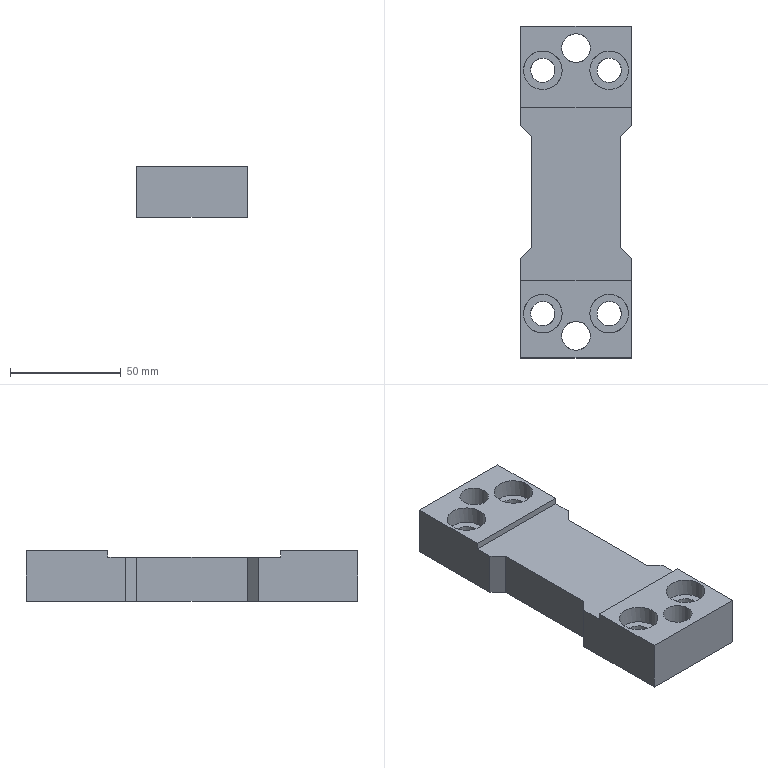Part | NX | features solid 2 | 1 solid | 32 faces | box 50 x 150 x 23 mm | volume 130295 mm3 | plane 22 | cylinder 10 | commonest cylinder face diameters 11 x4 17.5 x4 13 x2
STEP:
#1=CARTESIAN_POINT('',(-470.,-708.,-75.));
#2=VERTEX_POINT('',#1);
#3=CARTESIAN_POINT('',(-470.,-663.,-75.));
#4=VERTEX_POINT('',#3);
#5=CARTESIAN_POINT('',(-470.,-708.,-75.));
#6=DIRECTION('',(0.,1.,0.));
#7=VECTOR('',#6,1000.);
#8=LINE('',#5,#7);
#9=EDGE_CURVE('',#2,#4,#8,.T.);
#10=ORIENTED_EDGE('',*,*,#9,.F.);
#11=CARTESIAN_POINT('',(-520.,-708.,-75.));
#12=VERTEX_POINT('',#11);
#13=CARTESIAN_POINT('',(-520.,-708.,-75.));
#14=DIRECTION('',(1.,0.,0.));
#15=VECTOR('',#14,1000.);
#16=LINE('',#13,#15);
#17=EDGE_CURVE('',#12,#2,#16,.T.);
#18=ORIENTED_EDGE('',*,*,#17,.F.);
#19=CARTESIAN_POINT('',(-520.,-663.,-75.));
#20=VERTEX_POINT('',#19);
#21=CARTESIAN_POINT('',(-520.,-708.,-75.));
#22=DIRECTION('',(0.,1.,0.));
#23=VECTOR('',#22,1000.);
#24=LINE('',#21,#23);
#25=EDGE_CURVE('',#12,#20,#24,.T.);
#26=ORIENTED_EDGE('',*,*,#25,.T.);
#27=CARTESIAN_POINT('',(-515.,-658.,-75.));
#28=VERTEX_POINT('',#27);
#29=CARTESIAN_POINT('',(-515.,-658.,-75.));
#30=DIRECTION('',(-0.7071,-0.7071,0.));
#31=VECTOR('',#30,1000.);
#32=LINE('',#29,#31);
#33=EDGE_CURVE('',#28,#20,#32,.T.);
#34=ORIENTED_EDGE('',*,*,#33,.F.);
#35=CARTESIAN_POINT('',(-515.,-608.,-75.));
#36=VERTEX_POINT('',#35);
#37=CARTESIAN_POINT('',(-515.,-658.,-75.));
#38=DIRECTION('',(0.,1.,0.));
#39=VECTOR('',#38,1000.);
#40=LINE('',#37,#39);
#41=EDGE_CURVE('',#28,#36,#40,.T.);
#42=ORIENTED_EDGE('',*,*,#41,.T.);
#43=CARTESIAN_POINT('',(-520.,-603.,-75.));
#44=VERTEX_POINT('',#43);
#45=CARTESIAN_POINT('',(-515.,-608.,-75.));
#46=DIRECTION('',(-0.7071,0.7071,0.));
#47=VECTOR('',#46,1000.);
#48=LINE('',#45,#47);
#49=EDGE_CURVE('',#36,#44,#48,.T.);
#50=ORIENTED_EDGE('',*,*,#49,.T.);
#51=CARTESIAN_POINT('',(-520.,-558.,-75.));
#52=VERTEX_POINT('',#51);
#53=CARTESIAN_POINT('',(-520.,-603.,-75.));
#54=DIRECTION('',(0.,1.,0.));
#55=VECTOR('',#54,1000.);
#56=LINE('',#53,#55);
#57=EDGE_CURVE('',#44,#52,#56,.T.);
#58=ORIENTED_EDGE('',*,*,#57,.T.);
#59=CARTESIAN_POINT('',(-470.,-558.,-75.));
#60=VERTEX_POINT('',#59);
#61=CARTESIAN_POINT('',(-470.,-558.,-75.));
#62=DIRECTION('',(-1.,0.,0.));
#63=VECTOR('',#62,1000.);
#64=LINE('',#61,#63);
#65=EDGE_CURVE('',#60,#52,#64,.T.);
#66=ORIENTED_EDGE('',*,*,#65,.F.);
#67=CARTESIAN_POINT('',(-470.,-603.,-75.));
#68=VERTEX_POINT('',#67);
#69=CARTESIAN_POINT('',(-470.,-603.,-75.));
#70=DIRECTION('',(0.,1.,0.));
#71=VECTOR('',#70,1000.);
#72=LINE('',#69,#71);
#73=EDGE_CURVE('',#68,#60,#72,.T.);
#74=ORIENTED_EDGE('',*,*,#73,.F.);
#75=CARTESIAN_POINT('',(-475.,-608.,-75.));
#76=VERTEX_POINT('',#75);
#77=CARTESIAN_POINT('',(-475.,-608.,-75.));
#78=DIRECTION('',(0.7071,0.7071,0.));
#79=VECTOR('',#78,1000.);
#80=LINE('',#77,#79);
#81=EDGE_CURVE('',#76,#68,#80,.T.);
#82=ORIENTED_EDGE('',*,*,#81,.F.);
#83=CARTESIAN_POINT('',(-475.,-658.,-75.));
#84=VERTEX_POINT('',#83);
#85=CARTESIAN_POINT('',(-475.,-658.,-75.));
#86=DIRECTION('',(0.,1.,0.));
#87=VECTOR('',#86,1000.);
#88=LINE('',#85,#87);
#89=EDGE_CURVE('',#84,#76,#88,.T.);
#90=ORIENTED_EDGE('',*,*,#89,.F.);
#91=CARTESIAN_POINT('',(-470.,-663.,-75.));
#92=DIRECTION('',(-0.7071,0.7071,0.));
#93=VECTOR('',#92,1000.);
#94=LINE('',#91,#93);
#95=EDGE_CURVE('',#4,#84,#94,.T.);
#96=ORIENTED_EDGE('',*,*,#95,.F.);
#97=EDGE_LOOP('',(#10,#18,#26,#34,#42,#50,#58,#66,#74,#82,#90,#96));
#98=FACE_BOUND('',#97,.T.);
#99=CARTESIAN_POINT('',(-510.,-682.5,-75.));
#100=VERTEX_POINT('',#99);
#101=CARTESIAN_POINT('',(-510.,-688.,-75.));
#102=DIRECTION('',(0.,0.,-1.));
#103=DIRECTION('',(0.,1.,0.));
#104=AXIS2_PLACEMENT_3D('',#101,#102,#103);
#105=CIRCLE('',#104,5.5);
#106=EDGE_CURVE('',#100,#100,#105,.T.);
#107=ORIENTED_EDGE('',*,*,#106,.F.);
#108=EDGE_LOOP('',(#107));
#109=FACE_BOUND('',#108,.T.);
#110=CARTESIAN_POINT('',(-480.,-682.5,-75.));
#111=VERTEX_POINT('',#110);
#112=CARTESIAN_POINT('',(-480.,-688.,-75.));
#113=DIRECTION('',(0.,0.,-1.));
#114=DIRECTION('',(0.,1.,0.));
#115=AXIS2_PLACEMENT_3D('',#112,#113,#114);
#116=CIRCLE('',#115,5.5);
#117=EDGE_CURVE('',#111,#111,#116,.T.);
#118=ORIENTED_EDGE('',*,*,#117,.F.);
#119=EDGE_LOOP('',(#118));
#120=FACE_BOUND('',#119,.T.);
#121=CARTESIAN_POINT('',(-495.,-691.5,-75.));
#122=VERTEX_POINT('',#121);
#123=CARTESIAN_POINT('',(-495.,-698.,-75.));
#124=DIRECTION('',(0.,0.,-1.));
#125=DIRECTION('',(0.,1.,0.));
#126=AXIS2_PLACEMENT_3D('',#123,#124,#125);
#127=CIRCLE('',#126,6.5);
#128=EDGE_CURVE('',#122,#122,#127,.T.);
#129=ORIENTED_EDGE('',*,*,#128,.F.);
#130=EDGE_LOOP('',(#129));
#131=FACE_BOUND('',#130,.T.);
#132=CARTESIAN_POINT('',(-495.,-561.5,-75.));
#133=VERTEX_POINT('',#132);
#134=CARTESIAN_POINT('',(-495.,-568.,-75.));
#135=DIRECTION('',(0.,0.,-1.));
#136=DIRECTION('',(0.,1.,0.));
#137=AXIS2_PLACEMENT_3D('',#134,#135,#136);
#138=CIRCLE('',#137,6.5);
#139=EDGE_CURVE('',#133,#133,#138,.T.);
#140=ORIENTED_EDGE('',*,*,#139,.F.);
#141=EDGE_LOOP('',(#140));
#142=FACE_BOUND('',#141,.T.);
#143=CARTESIAN_POINT('',(-480.,-572.5,-75.));
#144=VERTEX_POINT('',#143);
#145=CARTESIAN_POINT('',(-480.,-578.,-75.));
#146=DIRECTION('',(0.,0.,-1.));
#147=DIRECTION('',(0.,1.,0.));
#148=AXIS2_PLACEMENT_3D('',#145,#146,#147);
#149=CIRCLE('',#148,5.5);
#150=EDGE_CURVE('',#144,#144,#149,.T.);
#151=ORIENTED_EDGE('',*,*,#150,.F.);
#152=EDGE_LOOP('',(#151));
#153=FACE_BOUND('',#152,.T.);
#154=CARTESIAN_POINT('',(-510.,-572.5,-75.));
#155=VERTEX_POINT('',#154);
#156=CARTESIAN_POINT('',(-510.,-578.,-75.));
#157=DIRECTION('',(0.,0.,-1.));
#158=DIRECTION('',(0.,1.,0.));
#159=AXIS2_PLACEMENT_3D('',#156,#157,#158);
#160=CIRCLE('',#159,5.5);
#161=EDGE_CURVE('',#155,#155,#160,.T.);
#162=ORIENTED_EDGE('',*,*,#161,.F.);
#163=EDGE_LOOP('',(#162));
#164=FACE_BOUND('',#163,.T.);
#165=CARTESIAN_POINT('',(-470.,-708.,-75.));
#166=DIRECTION('',(0.,0.,-1.));
#167=DIRECTION('',(1.,0.,0.));
#168=AXIS2_PLACEMENT_3D('',#165,#166,#167);
#169=PLANE('',#168);
#170=ADVANCED_FACE('',(#98,#109,#120,#131,#142,#153,#164),#169,.T.);
#171=CARTESIAN_POINT('',(-470.,-673.,-52.));
#172=VERTEX_POINT('',#171);
#173=CARTESIAN_POINT('',(-470.,-673.,-55.));
#174=VERTEX_POINT('',#173);
#175=CARTESIAN_POINT('',(-470.,-673.,-54.));
#176=DIRECTION('',(0.,0.,-1.));
#177=VECTOR('',#176,1000.);
#178=LINE('',#175,#177);
#179=EDGE_CURVE('',#172,#174,#178,.T.);
#180=ORIENTED_EDGE('',*,*,#179,.F.);
#181=CARTESIAN_POINT('',(-470.,-708.,-52.));
#182=VERTEX_POINT('',#181);
#183=CARTESIAN_POINT('',(-470.,-708.,-52.));
#184=DIRECTION('',(0.,1.,0.));
#185=VECTOR('',#184,1000.);
#186=LINE('',#183,#185);
#187=EDGE_CURVE('',#182,#172,#186,.T.);
#188=ORIENTED_EDGE('',*,*,#187,.F.);
#189=CARTESIAN_POINT('',(-470.,-708.,-54.));
#190=DIRECTION('',(0.,0.,-1.));
#191=VECTOR('',#190,1000.);
#192=LINE('',#189,#191);
#193=EDGE_CURVE('',#182,#2,#192,.T.);
#194=ORIENTED_EDGE('',*,*,#193,.T.);
#195=ORIENTED_EDGE('',*,*,#9,.T.);
#196=CARTESIAN_POINT('',(-470.,-663.,-55.));
#197=VERTEX_POINT('',#196);
#198=CARTESIAN_POINT('',(-470.,-663.,-54.));
#199=DIRECTION('',(0.,0.,-1.));
#200=VECTOR('',#199,1000.);
#201=LINE('',#198,#200);
#202=EDGE_CURVE('',#197,#4,#201,.T.);
#203=ORIENTED_EDGE('',*,*,#202,.F.);
#204=CARTESIAN_POINT('',(-470.,-708.,-55.));
#205=DIRECTION('',(0.,1.,0.));
#206=VECTOR('',#205,1000.);
#207=LINE('',#204,#206);
#208=EDGE_CURVE('',#174,#197,#207,.T.);
#209=ORIENTED_EDGE('',*,*,#208,.F.);
#210=EDGE_LOOP('',(#180,#188,#194,#195,#203,#209));
#211=FACE_BOUND('',#210,.T.);
#212=CARTESIAN_POINT('',(-470.,-708.,-54.));
#213=DIRECTION('',(1.,0.,0.));
#214=DIRECTION('',(0.,-1.,0.));
#215=AXIS2_PLACEMENT_3D('',#212,#213,#214);
#216=PLANE('',#215);
#217=ADVANCED_FACE('',(#211),#216,.T.);
#218=ORIENTED_EDGE('',*,*,#25,.F.);
#219=CARTESIAN_POINT('',(-520.,-708.,-52.));
#220=VERTEX_POINT('',#219);
#221=CARTESIAN_POINT('',(-520.,-708.,-54.));
#222=DIRECTION('',(0.,0.,-1.));
#223=VECTOR('',#222,1000.);
#224=LINE('',#221,#223);
#225=EDGE_CURVE('',#220,#12,#224,.T.);
#226=ORIENTED_EDGE('',*,*,#225,.F.);
#227=CARTESIAN_POINT('',(-520.,-673.,-52.));
#228=VERTEX_POINT('',#227);
#229=CARTESIAN_POINT('',(-520.,-708.,-52.));
#230=DIRECTION('',(0.,1.,0.));
#231=VECTOR('',#230,1000.);
#232=LINE('',#229,#231);
#233=EDGE_CURVE('',#220,#228,#232,.T.);
#234=ORIENTED_EDGE('',*,*,#233,.T.);
#235=CARTESIAN_POINT('',(-520.,-673.,-55.));
#236=VERTEX_POINT('',#235);
#237=CARTESIAN_POINT('',(-520.,-673.,-54.));
#238=DIRECTION('',(0.,0.,1.));
#239=VECTOR('',#238,1000.);
#240=LINE('',#237,#239);
#241=EDGE_CURVE('',#236,#228,#240,.T.);
#242=ORIENTED_EDGE('',*,*,#241,.F.);
#243=CARTESIAN_POINT('',(-520.,-663.,-55.));
#244=VERTEX_POINT('',#243);
#245=CARTESIAN_POINT('',(-520.,-708.,-55.));
#246=DIRECTION('',(0.,1.,0.));
#247=VECTOR('',#246,1000.);
#248=LINE('',#245,#247);
#249=EDGE_CURVE('',#236,#244,#248,.T.);
#250=ORIENTED_EDGE('',*,*,#249,.T.);
#251=CARTESIAN_POINT('',(-520.,-663.,-54.));
#252=DIRECTION('',(0.,0.,-1.));
#253=VECTOR('',#252,1000.);
#254=LINE('',#251,#253);
#255=EDGE_CURVE('',#244,#20,#254,.T.);
#256=ORIENTED_EDGE('',*,*,#255,.T.);
#257=EDGE_LOOP('',(#218,#226,#234,#242,#250,#256));
#258=FACE_BOUND('',#257,.T.);
#259=CARTESIAN_POINT('',(-520.,-708.,-54.));
#260=DIRECTION('',(1.,0.,0.));
#261=DIRECTION('',(0.,-1.,0.));
#262=AXIS2_PLACEMENT_3D('',#259,#260,#261);
#263=PLANE('',#262);
#264=ADVANCED_FACE('',(#258),#263,.F.);
#265=CARTESIAN_POINT('',(-520.,-673.,-55.));
#266=DIRECTION('',(-1.,0.,0.));
#267=VECTOR('',#266,1000.);
#268=LINE('',#265,#267);
#269=EDGE_CURVE('',#174,#236,#268,.T.);
#270=ORIENTED_EDGE('',*,*,#269,.T.);
#271=ORIENTED_EDGE('',*,*,#241,.T.);
#272=CARTESIAN_POINT('',(-470.,-673.,-52.));
#273=DIRECTION('',(-1.,0.,0.));
#274=VECTOR('',#273,1000.);
#275=LINE('',#272,#274);
#276=EDGE_CURVE('',#172,#228,#275,.T.);
#277=ORIENTED_EDGE('',*,*,#276,.F.);
#278=ORIENTED_EDGE('',*,*,#179,.T.);
#279=EDGE_LOOP('',(#270,#271,#277,#278));
#280=FACE_BOUND('',#279,.T.);
#281=CARTESIAN_POINT('',(-470.,-673.,-35.44));
#282=DIRECTION('',(0.,1.,0.));
#283=DIRECTION('',(1.,0.,0.));
#284=AXIS2_PLACEMENT_3D('',#281,#282,#283);
#285=PLANE('',#284);
#286=ADVANCED_FACE('',(#280),#285,.T.);
#287=CARTESIAN_POINT('',(-485.5,-688.,-60.));
#288=VERTEX_POINT('',#287);
#289=CARTESIAN_POINT('',(-480.,-688.,-60.));
#290=DIRECTION('',(0.,0.,-1.));
#291=DIRECTION('',(-1.,0.,0.));
#292=AXIS2_PLACEMENT_3D('',#289,#290,#291);
#293=CIRCLE('',#292,5.5);
#294=EDGE_CURVE('',#288,#288,#293,.T.);
#295=ORIENTED_EDGE('',*,*,#294,.T.);
#296=EDGE_LOOP('',(#295));
#297=FACE_BOUND('',#296,.T.);
#298=CARTESIAN_POINT('',(-480.,-679.25,-60.));
#299=VERTEX_POINT('',#298);
#300=CARTESIAN_POINT('',(-480.,-688.,-60.));
#301=DIRECTION('',(0.,0.,-1.));
#302=DIRECTION('',(0.,1.,0.));
#303=AXIS2_PLACEMENT_3D('',#300,#301,#302);
#304=CIRCLE('',#303,8.75);
#305=EDGE_CURVE('',#299,#299,#304,.T.);
#306=ORIENTED_EDGE('',*,*,#305,.F.);
#307=EDGE_LOOP('',(#306));
#308=FACE_BOUND('',#307,.T.);
#309=CARTESIAN_POINT('',(-480.,-688.,-60.));
#310=DIRECTION('',(0.,0.,1.));
#311=DIRECTION('',(-1.,0.,0.));
#312=AXIS2_PLACEMENT_3D('',#309,#310,#311);
#313=PLANE('',#312);
#314=ADVANCED_FACE('',(#297,#308),#313,.T.);
#315=CARTESIAN_POINT('',(-515.5,-688.,-60.));
#316=VERTEX_POINT('',#315);
#317=CARTESIAN_POINT('',(-510.,-688.,-60.));
#318=DIRECTION('',(0.,0.,-1.));
#319=DIRECTION('',(-1.,0.,0.));
#320=AXIS2_PLACEMENT_3D('',#317,#318,#319);
#321=CIRCLE('',#320,5.5);
#322=EDGE_CURVE('',#316,#316,#321,.T.);
#323=ORIENTED_EDGE('',*,*,#322,.T.);
#324=EDGE_LOOP('',(#323));
#325=FACE_BOUND('',#324,.T.);
#326=CARTESIAN_POINT('',(-510.,-679.25,-60.));
#327=VERTEX_POINT('',#326);
#328=CARTESIAN_POINT('',(-510.,-688.,-60.));
#329=DIRECTION('',(0.,0.,-1.));
#330=DIRECTION('',(0.,1.,0.));
#331=AXIS2_PLACEMENT_3D('',#328,#329,#330);
#332=CIRCLE('',#331,8.75);
#333=EDGE_CURVE('',#327,#327,#332,.T.);
#334=ORIENTED_EDGE('',*,*,#333,.F.);
#335=EDGE_LOOP('',(#334));
#336=FACE_BOUND('',#335,.T.);
#337=CARTESIAN_POINT('',(-510.,-688.,-60.));
#338=DIRECTION('',(0.,0.,1.));
#339=DIRECTION('',(-1.,0.,0.));
#340=AXIS2_PLACEMENT_3D('',#337,#338,#339);
#341=PLANE('',#340);
#342=ADVANCED_FACE('',(#325,#336),#341,.T.);
#343=CARTESIAN_POINT('',(-471.25,-688.,-52.));
#344=VERTEX_POINT('',#343);
#345=CARTESIAN_POINT('',(-480.,-688.,-52.));
#346=DIRECTION('',(0.,0.,1.));
#347=DIRECTION('',(1.,0.,0.));
#348=AXIS2_PLACEMENT_3D('',#345,#346,#347);
#349=CIRCLE('',#348,8.75);
#350=EDGE_CURVE('',#344,#344,#349,.F.);
#351=ORIENTED_EDGE('',*,*,#350,.F.);
#352=EDGE_LOOP('',(#351));
#353=FACE_BOUND('',#352,.T.);
#354=ORIENTED_EDGE('',*,*,#305,.T.);
#355=EDGE_LOOP('',(#354));
#356=FACE_BOUND('',#355,.T.);
#357=CARTESIAN_POINT('',(-480.,-688.,-54.));
#358=DIRECTION('',(0.,0.,-1.));
#359=DIRECTION('',(1.,0.,0.));
#360=AXIS2_PLACEMENT_3D('',#357,#358,#359);
#361=CYLINDRICAL_SURFACE('',#360,8.75);
#362=ADVANCED_FACE('',(#353,#356),#361,.F.);
#363=CARTESIAN_POINT('',(-501.25,-688.,-52.));
#364=VERTEX_POINT('',#363);
#365=CARTESIAN_POINT('',(-510.,-688.,-52.));
#366=DIRECTION('',(0.,0.,1.));
#367=DIRECTION('',(1.,0.,0.));
#368=AXIS2_PLACEMENT_3D('',#365,#366,#367);
#369=CIRCLE('',#368,8.75);
#370=EDGE_CURVE('',#364,#364,#369,.F.);
#371=ORIENTED_EDGE('',*,*,#370,.F.);
#372=EDGE_LOOP('',(#371));
#373=FACE_BOUND('',#372,.T.);
#374=ORIENTED_EDGE('',*,*,#333,.T.);
#375=EDGE_LOOP('',(#374));
#376=FACE_BOUND('',#375,.T.);
#377=CARTESIAN_POINT('',(-510.,-688.,-54.));
#378=DIRECTION('',(0.,0.,-1.));
#379=DIRECTION('',(1.,0.,0.));
#380=AXIS2_PLACEMENT_3D('',#377,#378,#379);
#381=CYLINDRICAL_SURFACE('',#380,8.75);
#382=ADVANCED_FACE('',(#373,#376),#381,.F.);
#383=CARTESIAN_POINT('',(-488.5,-698.,-52.));
#384=VERTEX_POINT('',#383);
#385=CARTESIAN_POINT('',(-495.,-698.,-52.));
#386=DIRECTION('',(0.,0.,1.));
#387=DIRECTION('',(1.,0.,0.));
#388=AXIS2_PLACEMENT_3D('',#385,#386,#387);
#389=CIRCLE('',#388,6.5);
#390=EDGE_CURVE('',#384,#384,#389,.F.);
#391=ORIENTED_EDGE('',*,*,#390,.F.);
#392=EDGE_LOOP('',(#391));
#393=FACE_BOUND('',#392,.T.);
#394=ORIENTED_EDGE('',*,*,#128,.T.);
#395=EDGE_LOOP('',(#394));
#396=FACE_BOUND('',#395,.T.);
#397=CARTESIAN_POINT('',(-495.,-698.,-54.));
#398=DIRECTION('',(0.,0.,-1.));
#399=DIRECTION('',(1.,0.,0.));
#400=AXIS2_PLACEMENT_3D('',#397,#398,#399);
#401=CYLINDRICAL_SURFACE('',#400,6.5);
#402=ADVANCED_FACE('',(#393,#396),#401,.F.);
#403=ORIENTED_EDGE('',*,*,#117,.T.);
#404=EDGE_LOOP('',(#403));
#405=FACE_BOUND('',#404,.T.);
#406=ORIENTED_EDGE('',*,*,#294,.F.);
#407=EDGE_LOOP('',(#406));
#408=FACE_BOUND('',#407,.T.);
#409=CARTESIAN_POINT('',(-480.,-688.,-54.));
#410=DIRECTION('',(0.,0.,-1.));
#411=DIRECTION('',(1.,0.,0.));
#412=AXIS2_PLACEMENT_3D('',#409,#410,#411);
#413=CYLINDRICAL_SURFACE('',#412,5.5);
#414=ADVANCED_FACE('',(#405,#408),#413,.F.);
#415=ORIENTED_EDGE('',*,*,#106,.T.);
#416=EDGE_LOOP('',(#415));
#417=FACE_BOUND('',#416,.T.);
#418=ORIENTED_EDGE('',*,*,#322,.F.);
#419=EDGE_LOOP('',(#418));
#420=FACE_BOUND('',#419,.T.);
#421=CARTESIAN_POINT('',(-510.,-688.,-54.));
#422=DIRECTION('',(0.,0.,-1.));
#423=DIRECTION('',(1.,0.,0.));
#424=AXIS2_PLACEMENT_3D('',#421,#422,#423);
#425=CYLINDRICAL_SURFACE('',#424,5.5);
#426=ADVANCED_FACE('',(#417,#420),#425,.F.);
#427=ORIENTED_EDGE('',*,*,#17,.T.);
#428=ORIENTED_EDGE('',*,*,#193,.F.);
#429=CARTESIAN_POINT('',(-470.,-708.,-52.));
#430=DIRECTION('',(1.,0.,0.));
#431=VECTOR('',#430,1000.);
#432=LINE('',#429,#431);
#433=EDGE_CURVE('',#220,#182,#432,.T.);
#434=ORIENTED_EDGE('',*,*,#433,.F.);
#435=ORIENTED_EDGE('',*,*,#225,.T.);
#436=EDGE_LOOP('',(#427,#428,#434,#435));
#437=FACE_BOUND('',#436,.T.);
#438=CARTESIAN_POINT('',(-520.,-708.,-54.));
#439=DIRECTION('',(0.,-1.,0.));
#440=DIRECTION('',(-1.,0.,0.));
#441=AXIS2_PLACEMENT_3D('',#438,#439,#440);
#442=PLANE('',#441);
#443=ADVANCED_FACE('',(#437),#442,.T.);
#444=ORIENTED_EDGE('',*,*,#370,.T.);
#445=EDGE_LOOP('',(#444));
#446=FACE_BOUND('',#445,.T.);
#447=ORIENTED_EDGE('',*,*,#390,.T.);
#448=EDGE_LOOP('',(#447));
#449=FACE_BOUND('',#448,.T.);
#450=ORIENTED_EDGE('',*,*,#350,.T.);
#451=EDGE_LOOP('',(#450));
#452=FACE_BOUND('',#451,.T.);
#453=ORIENTED_EDGE('',*,*,#276,.T.);
#454=ORIENTED_EDGE('',*,*,#233,.F.);
#455=ORIENTED_EDGE('',*,*,#433,.T.);
#456=ORIENTED_EDGE('',*,*,#187,.T.);
#457=EDGE_LOOP('',(#453,#454,#455,#456));
#458=FACE_BOUND('',#457,.T.);
#459=CARTESIAN_POINT('',(-470.,-708.,-52.));
#460=DIRECTION('',(0.,0.,-1.));
#461=DIRECTION('',(1.,0.,0.));
#462=AXIS2_PLACEMENT_3D('',#459,#460,#461);
#463=PLANE('',#462);
#464=ADVANCED_FACE('',(#446,#449,#452,#458),#463,.F.);
#465=ORIENTED_EDGE('',*,*,#49,.F.);
#466=CARTESIAN_POINT('',(-515.,-608.,-55.));
#467=VERTEX_POINT('',#466);
#468=CARTESIAN_POINT('',(-515.,-608.,-54.));
#469=DIRECTION('',(0.,0.,-1.));
#470=VECTOR('',#469,1000.);
#471=LINE('',#468,#470);
#472=EDGE_CURVE('',#467,#36,#471,.T.);
#473=ORIENTED_EDGE('',*,*,#472,.F.);
#474=CARTESIAN_POINT('',(-520.,-603.,-55.));
#475=VERTEX_POINT('',#474);
#476=CARTESIAN_POINT('',(-442.5,-680.5,-55.));
#477=DIRECTION('',(-0.7071,0.7071,0.));
#478=VECTOR('',#477,1000.);
#479=LINE('',#476,#478);
#480=EDGE_CURVE('',#467,#475,#479,.T.);
#481=ORIENTED_EDGE('',*,*,#480,.T.);
#482=CARTESIAN_POINT('',(-520.,-603.,-54.));
#483=DIRECTION('',(0.,0.,-1.));
#484=VECTOR('',#483,1000.);
#485=LINE('',#482,#484);
#486=EDGE_CURVE('',#475,#44,#485,.T.);
#487=ORIENTED_EDGE('',*,*,#486,.T.);
#488=EDGE_LOOP('',(#465,#473,#481,#487));
#489=FACE_BOUND('',#488,.T.);
#490=CARTESIAN_POINT('',(-515.,-608.,-54.));
#491=DIRECTION('',(0.7071,0.7071,0.));
#492=DIRECTION('',(0.7071,-0.7071,0.));
#493=AXIS2_PLACEMENT_3D('',#490,#491,#492);
#494=PLANE('',#493);
#495=ADVANCED_FACE('',(#489),#494,.F.);
#496=ORIENTED_EDGE('',*,*,#41,.F.);
#497=CARTESIAN_POINT('',(-515.,-658.,-55.));
#498=VERTEX_POINT('',#497);
#499=CARTESIAN_POINT('',(-515.,-658.,-54.));
#500=DIRECTION('',(0.,0.,-1.));
#501=VECTOR('',#500,1000.);
#502=LINE('',#499,#501);
#503=EDGE_CURVE('',#498,#28,#502,.T.);
#504=ORIENTED_EDGE('',*,*,#503,.F.);
#505=CARTESIAN_POINT('',(-515.,-708.,-55.));
#506=DIRECTION('',(0.,1.,0.));
#507=VECTOR('',#506,1000.);
#508=LINE('',#505,#507);
#509=EDGE_CURVE('',#498,#467,#508,.T.);
#510=ORIENTED_EDGE('',*,*,#509,.T.);
#511=ORIENTED_EDGE('',*,*,#472,.T.);
#512=EDGE_LOOP('',(#496,#504,#510,#511));
#513=FACE_BOUND('',#512,.T.);
#514=CARTESIAN_POINT('',(-515.,-658.,-54.));
#515=DIRECTION('',(1.,0.,0.));
#516=DIRECTION('',(0.,-1.,0.));
#517=AXIS2_PLACEMENT_3D('',#514,#515,#516);
#518=PLANE('',#517);
#519=ADVANCED_FACE('',(#513),#518,.F.);
#520=ORIENTED_EDGE('',*,*,#33,.T.);
#521=ORIENTED_EDGE('',*,*,#255,.F.);
#522=CARTESIAN_POINT('',(-517.5,-660.5,-55.));
#523=DIRECTION('',(-0.7071,-0.7071,0.));
#524=VECTOR('',#523,1000.);
#525=LINE('',#522,#524);
#526=EDGE_CURVE('',#498,#244,#525,.T.);
#527=ORIENTED_EDGE('',*,*,#526,.F.);
#528=ORIENTED_EDGE('',*,*,#503,.T.);
#529=EDGE_LOOP('',(#520,#521,#527,#528));
#530=FACE_BOUND('',#529,.T.);
#531=CARTESIAN_POINT('',(-515.,-658.,-54.));
#532=DIRECTION('',(-0.7071,0.7071,0.));
#533=DIRECTION('',(0.7071,0.7071,0.));
#534=AXIS2_PLACEMENT_3D('',#531,#532,#533);
#535=PLANE('',#534);
#536=ADVANCED_FACE('',(#530),#535,.T.);
#537=ORIENTED_EDGE('',*,*,#95,.T.);
#538=CARTESIAN_POINT('',(-475.,-658.,-55.));
#539=VERTEX_POINT('',#538);
#540=CARTESIAN_POINT('',(-475.,-658.,-54.));
#541=DIRECTION('',(0.,0.,-1.));
#542=VECTOR('',#541,1000.);
#543=LINE('',#540,#542);
#544=EDGE_CURVE('',#539,#84,#543,.T.);
#545=ORIENTED_EDGE('',*,*,#544,.F.);
#546=CARTESIAN_POINT('',(-447.5,-685.5,-55.));
#547=DIRECTION('',(-0.7071,0.7071,0.));
#548=VECTOR('',#547,1000.);
#549=LINE('',#546,#548);
#550=EDGE_CURVE('',#197,#539,#549,.T.);
#551=ORIENTED_EDGE('',*,*,#550,.F.);
#552=ORIENTED_EDGE('',*,*,#202,.T.);
#553=EDGE_LOOP('',(#537,#545,#551,#552));
#554=FACE_BOUND('',#553,.T.);
#555=CARTESIAN_POINT('',(-470.,-663.,-54.));
#556=DIRECTION('',(0.7071,0.7071,0.));
#557=DIRECTION('',(0.7071,-0.7071,0.));
#558=AXIS2_PLACEMENT_3D('',#555,#556,#557);
#559=PLANE('',#558);
#560=ADVANCED_FACE('',(#554),#559,.T.);
#561=ORIENTED_EDGE('',*,*,#89,.T.);
#562=CARTESIAN_POINT('',(-475.,-608.,-55.));
#563=VERTEX_POINT('',#562);
#564=CARTESIAN_POINT('',(-475.,-608.,-54.));
#565=DIRECTION('',(0.,0.,-1.));
#566=VECTOR('',#565,1000.);
#567=LINE('',#564,#566);
#568=EDGE_CURVE('',#563,#76,#567,.T.);
#569=ORIENTED_EDGE('',*,*,#568,.F.);
#570=CARTESIAN_POINT('',(-475.,-708.,-55.));
#571=DIRECTION('',(0.,1.,0.));
#572=VECTOR('',#571,1000.);
#573=LINE('',#570,#572);
#574=EDGE_CURVE('',#539,#563,#573,.T.);
#575=ORIENTED_EDGE('',*,*,#574,.F.);
#576=ORIENTED_EDGE('',*,*,#544,.T.);
#577=EDGE_LOOP('',(#561,#569,#575,#576));
#578=FACE_BOUND('',#577,.T.);
#579=CARTESIAN_POINT('',(-475.,-658.,-54.));
#580=DIRECTION('',(1.,0.,0.));
#581=DIRECTION('',(0.,-1.,0.));
#582=AXIS2_PLACEMENT_3D('',#579,#580,#581);
#583=PLANE('',#582);
#584=ADVANCED_FACE('',(#578),#583,.T.);
#585=ORIENTED_EDGE('',*,*,#81,.T.);
#586=CARTESIAN_POINT('',(-470.,-603.,-55.));
#587=VERTEX_POINT('',#586);
#588=CARTESIAN_POINT('',(-470.,-603.,-54.));
#589=DIRECTION('',(0.,0.,-1.));
#590=VECTOR('',#589,1000.);
#591=LINE('',#588,#590);
#592=EDGE_CURVE('',#587,#68,#591,.T.);
#593=ORIENTED_EDGE('',*,*,#592,.F.);
#594=CARTESIAN_POINT('',(-522.5,-655.5,-55.));
#595=DIRECTION('',(0.7071,0.7071,0.));
#596=VECTOR('',#595,1000.);
#597=LINE('',#594,#596);
#598=EDGE_CURVE('',#563,#587,#597,.T.);
#599=ORIENTED_EDGE('',*,*,#598,.F.);
#600=ORIENTED_EDGE('',*,*,#568,.T.);
#601=EDGE_LOOP('',(#585,#593,#599,#600));
#602=FACE_BOUND('',#601,.T.);
#603=CARTESIAN_POINT('',(-475.,-608.,-54.));
#604=DIRECTION('',(0.7071,-0.7071,0.));
#605=DIRECTION('',(-0.7071,-0.7071,0.));
#606=AXIS2_PLACEMENT_3D('',#603,#604,#605);
#607=PLANE('',#606);
#608=ADVANCED_FACE('',(#602),#607,.T.);
#609=CARTESIAN_POINT('',(-470.,-595.,-55.));
#610=VERTEX_POINT('',#609);
#611=CARTESIAN_POINT('',(-470.,-708.,-55.));
#612=DIRECTION('',(0.,1.,0.));
#613=VECTOR('',#612,1000.);
#614=LINE('',#611,#613);
#615=EDGE_CURVE('',#587,#610,#614,.T.);
#616=ORIENTED_EDGE('',*,*,#615,.F.);
#617=ORIENTED_EDGE('',*,*,#592,.T.);
#618=ORIENTED_EDGE('',*,*,#73,.T.);
#619=CARTESIAN_POINT('',(-470.,-558.,-52.));
#620=VERTEX_POINT('',#619);
#621=CARTESIAN_POINT('',(-470.,-558.,-54.));
#622=DIRECTION('',(0.,0.,-1.));
#623=VECTOR('',#622,1000.);
#624=LINE('',#621,#623);
#625=EDGE_CURVE('',#620,#60,#624,.T.);
#626=ORIENTED_EDGE('',*,*,#625,.F.);
#627=CARTESIAN_POINT('',(-470.,-595.,-52.));
#628=VERTEX_POINT('',#627);
#629=CARTESIAN_POINT('',(-470.,-708.,-52.));
#630=DIRECTION('',(0.,1.,0.));
#631=VECTOR('',#630,1000.);
#632=LINE('',#629,#631);
#633=EDGE_CURVE('',#628,#620,#632,.T.);
#634=ORIENTED_EDGE('',*,*,#633,.F.);
#635=CARTESIAN_POINT('',(-470.,-595.,-54.));
#636=DIRECTION('',(0.,0.,1.));
#637=VECTOR('',#636,1000.);
#638=LINE('',#635,#637);
#639=EDGE_CURVE('',#610,#628,#638,.T.);
#640=ORIENTED_EDGE('',*,*,#639,.F.);
#641=EDGE_LOOP('',(#616,#617,#618,#626,#634,#640));
#642=FACE_BOUND('',#641,.T.);
#643=CARTESIAN_POINT('',(-470.,-603.,-54.));
#644=DIRECTION('',(1.,0.,0.));
#645=DIRECTION('',(0.,-1.,0.));
#646=AXIS2_PLACEMENT_3D('',#643,#644,#645);
#647=PLANE('',#646);
#648=ADVANCED_FACE('',(#642),#647,.T.);
#649=ORIENTED_EDGE('',*,*,#57,.F.);
#650=ORIENTED_EDGE('',*,*,#486,.F.);
#651=CARTESIAN_POINT('',(-520.,-595.,-55.));
#652=VERTEX_POINT('',#651);
#653=CARTESIAN_POINT('',(-520.,-708.,-55.));
#654=DIRECTION('',(0.,1.,0.));
#655=VECTOR('',#654,1000.);
#656=LINE('',#653,#655);
#657=EDGE_CURVE('',#475,#652,#656,.T.);
#658=ORIENTED_EDGE('',*,*,#657,.T.);
#659=CARTESIAN_POINT('',(-520.,-595.,-52.));
#660=VERTEX_POINT('',#659);
#661=CARTESIAN_POINT('',(-520.,-595.,-54.));
#662=DIRECTION('',(0.,0.,1.));
#663=VECTOR('',#662,1000.);
#664=LINE('',#661,#663);
#665=EDGE_CURVE('',#652,#660,#664,.T.);
#666=ORIENTED_EDGE('',*,*,#665,.T.);
#667=CARTESIAN_POINT('',(-520.,-558.,-52.));
#668=VERTEX_POINT('',#667);
#669=CARTESIAN_POINT('',(-520.,-708.,-52.));
#670=DIRECTION('',(0.,1.,0.));
#671=VECTOR('',#670,1000.);
#672=LINE('',#669,#671);
#673=EDGE_CURVE('',#660,#668,#672,.T.);
#674=ORIENTED_EDGE('',*,*,#673,.T.);
#675=CARTESIAN_POINT('',(-520.,-558.,-54.));
#676=DIRECTION('',(0.,0.,-1.));
#677=VECTOR('',#676,1000.);
#678=LINE('',#675,#677);
#679=EDGE_CURVE('',#668,#52,#678,.T.);
#680=ORIENTED_EDGE('',*,*,#679,.T.);
#681=EDGE_LOOP('',(#649,#650,#658,#666,#674,#680));
#682=FACE_BOUND('',#681,.T.);
#683=CARTESIAN_POINT('',(-520.,-603.,-54.));
#684=DIRECTION('',(1.,0.,0.));
#685=DIRECTION('',(0.,-1.,0.));
#686=AXIS2_PLACEMENT_3D('',#683,#684,#685);
#687=PLANE('',#686);
#688=ADVANCED_FACE('',(#682),#687,.F.);
#689=ORIENTED_EDGE('',*,*,#657,.F.);
#690=ORIENTED_EDGE('',*,*,#480,.F.);
#691=ORIENTED_EDGE('',*,*,#509,.F.);
#692=ORIENTED_EDGE('',*,*,#526,.T.);
#693=ORIENTED_EDGE('',*,*,#249,.F.);
#694=ORIENTED_EDGE('',*,*,#269,.F.);
#695=ORIENTED_EDGE('',*,*,#208,.T.);
#696=ORIENTED_EDGE('',*,*,#550,.T.);
#697=ORIENTED_EDGE('',*,*,#574,.T.);
#698=ORIENTED_EDGE('',*,*,#598,.T.);
#699=ORIENTED_EDGE('',*,*,#615,.T.);
#700=CARTESIAN_POINT('',(-470.,-595.,-55.));
#701=DIRECTION('',(1.,0.,0.));
#702=VECTOR('',#701,1000.);
#703=LINE('',#700,#702);
#704=EDGE_CURVE('',#652,#610,#703,.T.);
#705=ORIENTED_EDGE('',*,*,#704,.F.);
#706=EDGE_LOOP('',(#689,#690,#691,#692,#693,#694,#695,#696,#697,#698,#699,#705));
#707=FACE_BOUND('',#706,.T.);
#708=CARTESIAN_POINT('',(-470.,-708.,-55.));
#709=DIRECTION('',(0.,0.,-1.));
#710=DIRECTION('',(1.,0.,0.));
#711=AXIS2_PLACEMENT_3D('',#708,#709,#710);
#712=PLANE('',#711);
#713=ADVANCED_FACE('',(#707),#712,.F.);
#714=ORIENTED_EDGE('',*,*,#704,.T.);
#715=ORIENTED_EDGE('',*,*,#639,.T.);
#716=CARTESIAN_POINT('',(-470.,-595.,-52.));
#717=DIRECTION('',(1.,0.,0.));
#718=VECTOR('',#717,1000.);
#719=LINE('',#716,#718);
#720=EDGE_CURVE('',#660,#628,#719,.T.);
#721=ORIENTED_EDGE('',*,*,#720,.F.);
#722=ORIENTED_EDGE('',*,*,#665,.F.);
#723=EDGE_LOOP('',(#714,#715,#721,#722));
#724=FACE_BOUND('',#723,.T.);
#725=CARTESIAN_POINT('',(-507.,-595.,-47.));
#726=DIRECTION('',(0.,-1.,0.));
#727=DIRECTION('',(-1.,0.,0.));
#728=AXIS2_PLACEMENT_3D('',#725,#726,#727);
#729=PLANE('',#728);
#730=ADVANCED_FACE('',(#724),#729,.T.);
#731=CARTESIAN_POINT('',(-515.5,-578.,-60.));
#732=VERTEX_POINT('',#731);
#733=CARTESIAN_POINT('',(-510.,-578.,-60.));
#734=DIRECTION('',(0.,0.,-1.));
#735=DIRECTION('',(-1.,0.,0.));
#736=AXIS2_PLACEMENT_3D('',#733,#734,#735);
#737=CIRCLE('',#736,5.5);
#738=EDGE_CURVE('',#732,#732,#737,.T.);
#739=ORIENTED_EDGE('',*,*,#738,.T.);
#740=EDGE_LOOP('',(#739));
#741=FACE_BOUND('',#740,.T.);
#742=CARTESIAN_POINT('',(-510.,-569.25,-60.));
#743=VERTEX_POINT('',#742);
#744=CARTESIAN_POINT('',(-510.,-578.,-60.));
#745=DIRECTION('',(0.,0.,-1.));
#746=DIRECTION('',(0.,1.,0.));
#747=AXIS2_PLACEMENT_3D('',#744,#745,#746);
#748=CIRCLE('',#747,8.75);
#749=EDGE_CURVE('',#743,#743,#748,.T.);
#750=ORIENTED_EDGE('',*,*,#749,.F.);
#751=EDGE_LOOP('',(#750));
#752=FACE_BOUND('',#751,.T.);
#753=CARTESIAN_POINT('',(-510.,-578.,-60.));
#754=DIRECTION('',(0.,0.,1.));
#755=DIRECTION('',(-1.,0.,0.));
#756=AXIS2_PLACEMENT_3D('',#753,#754,#755);
#757=PLANE('',#756);
#758=ADVANCED_FACE('',(#741,#752),#757,.T.);
#759=CARTESIAN_POINT('',(-485.5,-578.,-60.));
#760=VERTEX_POINT('',#759);
#761=CARTESIAN_POINT('',(-480.,-578.,-60.));
#762=DIRECTION('',(0.,0.,-1.));
#763=DIRECTION('',(-1.,0.,0.));
#764=AXIS2_PLACEMENT_3D('',#761,#762,#763);
#765=CIRCLE('',#764,5.5);
#766=EDGE_CURVE('',#760,#760,#765,.T.);
#767=ORIENTED_EDGE('',*,*,#766,.T.);
#768=EDGE_LOOP('',(#767));
#769=FACE_BOUND('',#768,.T.);
#770=CARTESIAN_POINT('',(-480.,-569.25,-60.));
#771=VERTEX_POINT('',#770);
#772=CARTESIAN_POINT('',(-480.,-578.,-60.));
#773=DIRECTION('',(0.,0.,-1.));
#774=DIRECTION('',(0.,1.,0.));
#775=AXIS2_PLACEMENT_3D('',#772,#773,#774);
#776=CIRCLE('',#775,8.75);
#777=EDGE_CURVE('',#771,#771,#776,.T.);
#778=ORIENTED_EDGE('',*,*,#777,.F.);
#779=EDGE_LOOP('',(#778));
#780=FACE_BOUND('',#779,.T.);
#781=CARTESIAN_POINT('',(-480.,-578.,-60.));
#782=DIRECTION('',(0.,0.,1.));
#783=DIRECTION('',(-1.,0.,0.));
#784=AXIS2_PLACEMENT_3D('',#781,#782,#783);
#785=PLANE('',#784);
#786=ADVANCED_FACE('',(#769,#780),#785,.T.);
#787=CARTESIAN_POINT('',(-471.25,-578.,-52.));
#788=VERTEX_POINT('',#787);
#789=CARTESIAN_POINT('',(-480.,-578.,-52.));
#790=DIRECTION('',(0.,0.,1.));
#791=DIRECTION('',(1.,0.,0.));
#792=AXIS2_PLACEMENT_3D('',#789,#790,#791);
#793=CIRCLE('',#792,8.75);
#794=EDGE_CURVE('',#788,#788,#793,.F.);
#795=ORIENTED_EDGE('',*,*,#794,.F.);
#796=EDGE_LOOP('',(#795));
#797=FACE_BOUND('',#796,.T.);
#798=ORIENTED_EDGE('',*,*,#777,.T.);
#799=EDGE_LOOP('',(#798));
#800=FACE_BOUND('',#799,.T.);
#801=CARTESIAN_POINT('',(-480.,-578.,-54.));
#802=DIRECTION('',(0.,0.,-1.));
#803=DIRECTION('',(1.,0.,0.));
#804=AXIS2_PLACEMENT_3D('',#801,#802,#803);
#805=CYLINDRICAL_SURFACE('',#804,8.75);
#806=ADVANCED_FACE('',(#797,#800),#805,.F.);
#807=CARTESIAN_POINT('',(-501.25,-578.,-52.));
#808=VERTEX_POINT('',#807);
#809=CARTESIAN_POINT('',(-510.,-578.,-52.));
#810=DIRECTION('',(0.,0.,1.));
#811=DIRECTION('',(1.,0.,0.));
#812=AXIS2_PLACEMENT_3D('',#809,#810,#811);
#813=CIRCLE('',#812,8.75);
#814=EDGE_CURVE('',#808,#808,#813,.F.);
#815=ORIENTED_EDGE('',*,*,#814,.F.);
#816=EDGE_LOOP('',(#815));
#817=FACE_BOUND('',#816,.T.);
#818=ORIENTED_EDGE('',*,*,#749,.T.);
#819=EDGE_LOOP('',(#818));
#820=FACE_BOUND('',#819,.T.);
#821=CARTESIAN_POINT('',(-510.,-578.,-54.));
#822=DIRECTION('',(0.,0.,-1.));
#823=DIRECTION('',(1.,0.,0.));
#824=AXIS2_PLACEMENT_3D('',#821,#822,#823);
#825=CYLINDRICAL_SURFACE('',#824,8.75);
#826=ADVANCED_FACE('',(#817,#820),#825,.F.);
#827=ORIENTED_EDGE('',*,*,#161,.T.);
#828=EDGE_LOOP('',(#827));
#829=FACE_BOUND('',#828,.T.);
#830=ORIENTED_EDGE('',*,*,#738,.F.);
#831=EDGE_LOOP('',(#830));
#832=FACE_BOUND('',#831,.T.);
#833=CARTESIAN_POINT('',(-510.,-578.,-54.));
#834=DIRECTION('',(0.,0.,-1.));
#835=DIRECTION('',(1.,0.,0.));
#836=AXIS2_PLACEMENT_3D('',#833,#834,#835);
#837=CYLINDRICAL_SURFACE('',#836,5.5);
#838=ADVANCED_FACE('',(#829,#832),#837,.F.);
#839=ORIENTED_EDGE('',*,*,#150,.T.);
#840=EDGE_LOOP('',(#839));
#841=FACE_BOUND('',#840,.T.);
#842=ORIENTED_EDGE('',*,*,#766,.F.);
#843=EDGE_LOOP('',(#842));
#844=FACE_BOUND('',#843,.T.);
#845=CARTESIAN_POINT('',(-480.,-578.,-54.));
#846=DIRECTION('',(0.,0.,-1.));
#847=DIRECTION('',(1.,0.,0.));
#848=AXIS2_PLACEMENT_3D('',#845,#846,#847);
#849=CYLINDRICAL_SURFACE('',#848,5.5);
#850=ADVANCED_FACE('',(#841,#844),#849,.F.);
#851=CARTESIAN_POINT('',(-488.5,-568.,-52.));
#852=VERTEX_POINT('',#851);
#853=CARTESIAN_POINT('',(-495.,-568.,-52.));
#854=DIRECTION('',(0.,0.,1.));
#855=DIRECTION('',(1.,0.,0.));
#856=AXIS2_PLACEMENT_3D('',#853,#854,#855);
#857=CIRCLE('',#856,6.5);
#858=EDGE_CURVE('',#852,#852,#857,.F.);
#859=ORIENTED_EDGE('',*,*,#858,.F.);
#860=EDGE_LOOP('',(#859));
#861=FACE_BOUND('',#860,.T.);
#862=ORIENTED_EDGE('',*,*,#139,.T.);
#863=EDGE_LOOP('',(#862));
#864=FACE_BOUND('',#863,.T.);
#865=CARTESIAN_POINT('',(-495.,-568.,-54.));
#866=DIRECTION('',(0.,0.,-1.));
#867=DIRECTION('',(1.,0.,0.));
#868=AXIS2_PLACEMENT_3D('',#865,#866,#867);
#869=CYLINDRICAL_SURFACE('',#868,6.5);
#870=ADVANCED_FACE('',(#861,#864),#869,.F.);
#871=ORIENTED_EDGE('',*,*,#65,.T.);
#872=ORIENTED_EDGE('',*,*,#679,.F.);
#873=CARTESIAN_POINT('',(-470.,-558.,-52.));
#874=DIRECTION('',(-1.,0.,0.));
#875=VECTOR('',#874,1000.);
#876=LINE('',#873,#875);
#877=EDGE_CURVE('',#620,#668,#876,.T.);
#878=ORIENTED_EDGE('',*,*,#877,.F.);
#879=ORIENTED_EDGE('',*,*,#625,.T.);
#880=EDGE_LOOP('',(#871,#872,#878,#879));
#881=FACE_BOUND('',#880,.T.);
#882=CARTESIAN_POINT('',(-470.,-558.,-54.));
#883=DIRECTION('',(0.,1.,0.));
#884=DIRECTION('',(1.,0.,0.));
#885=AXIS2_PLACEMENT_3D('',#882,#883,#884);
#886=PLANE('',#885);
#887=ADVANCED_FACE('',(#881),#886,.T.);
#888=ORIENTED_EDGE('',*,*,#814,.T.);
#889=EDGE_LOOP('',(#888));
#890=FACE_BOUND('',#889,.T.);
#891=ORIENTED_EDGE('',*,*,#858,.T.);
#892=EDGE_LOOP('',(#891));
#893=FACE_BOUND('',#892,.T.);
#894=ORIENTED_EDGE('',*,*,#794,.T.);
#895=EDGE_LOOP('',(#894));
#896=FACE_BOUND('',#895,.T.);
#897=ORIENTED_EDGE('',*,*,#720,.T.);
#898=ORIENTED_EDGE('',*,*,#633,.T.);
#899=ORIENTED_EDGE('',*,*,#877,.T.);
#900=ORIENTED_EDGE('',*,*,#673,.F.);
#901=EDGE_LOOP('',(#897,#898,#899,#900));
#902=FACE_BOUND('',#901,.T.);
#903=CARTESIAN_POINT('',(-470.,-708.,-52.));
#904=DIRECTION('',(0.,0.,-1.));
#905=DIRECTION('',(1.,0.,0.));
#906=AXIS2_PLACEMENT_3D('',#903,#904,#905);
#907=PLANE('',#906);
#908=ADVANCED_FACE('',(#890,#893,#896,#902),#907,.F.);
#909=CLOSED_SHELL('',(#170,#217,#264,#286,#314,#342,#362,#382,#402,#414,#426,#443,#464,#495,#519,#536,#560,#584,#608,#648,#688,#713,#730,#758,#786,#806,#826,#838,#850,#870,#887,#908));
#910=MANIFOLD_SOLID_BREP('',#909);
#911=(LENGTH_UNIT()NAMED_UNIT(*)SI_UNIT(.MILLI.,.METRE.));
#912=UNCERTAINTY_MEASURE_WITH_UNIT(LENGTH_MEASURE(0.00001),#911,'','');
#913=(NAMED_UNIT(*)PLANE_ANGLE_UNIT()SI_UNIT($,.RADIAN.));
#914=(NAMED_UNIT(*)SI_UNIT($,.STERADIAN.)SOLID_ANGLE_UNIT());
#915=(GEOMETRIC_REPRESENTATION_CONTEXT(3)GLOBAL_UNCERTAINTY_ASSIGNED_CONTEXT((#912))GLOBAL_UNIT_ASSIGNED_CONTEXT((#911,#913,#914))REPRESENTATION_CONTEXT('',''));
#916=ADVANCED_BREP_SHAPE_REPRESENTATION('',(#910),#915);